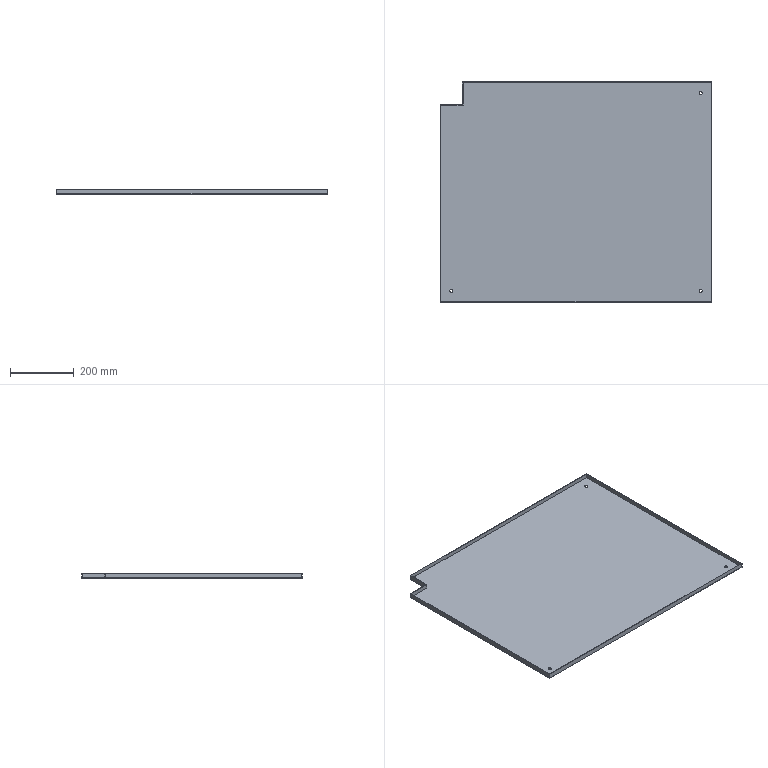Part | STEP file | 11-FGJJ-01211 | 1 solid | 21 faces | box 850 x 688 x 15 mm | volume 1239097 mm3 | plane 15 | cylinder 6 | commonest cylinder face diameters 10 x6
STEP:
#1=CARTESIAN_POINT('',(385.,-309.,2.));
#2=VERTEX_POINT('',#1);
#3=CARTESIAN_POINT('',(395.,-309.,2.));
#4=VERTEX_POINT('',#3);
#5=CARTESIAN_POINT('',(390.,-309.,2.));
#6=DIRECTION('',(0.,0.,1.));
#7=DIRECTION('',(1.,0.,0.));
#8=AXIS2_PLACEMENT_3D('',#5,#6,#7);
#9=CIRCLE('',#8,5.);
#10=EDGE_CURVE('',#2,#4,#9,.T.);
#11=ORIENTED_EDGE('',*,*,#10,.T.);
#12=CARTESIAN_POINT('',(395.,-309.,0.));
#13=VERTEX_POINT('',#12);
#14=CARTESIAN_POINT('',(395.,-309.,10.));
#15=DIRECTION('',(0.,0.,-1.));
#16=VECTOR('',#15,1000.);
#17=LINE('',#14,#16);
#18=EDGE_CURVE('',#4,#13,#17,.T.);
#19=ORIENTED_EDGE('',*,*,#18,.T.);
#20=CARTESIAN_POINT('',(385.,-309.,0.));
#21=VERTEX_POINT('',#20);
#22=CARTESIAN_POINT('',(390.,-309.,0.));
#23=DIRECTION('',(0.,0.,-1.));
#24=DIRECTION('',(-1.,0.,0.));
#25=AXIS2_PLACEMENT_3D('',#22,#23,#24);
#26=CIRCLE('',#25,5.);
#27=EDGE_CURVE('',#13,#21,#26,.T.);
#28=ORIENTED_EDGE('',*,*,#27,.T.);
#29=CARTESIAN_POINT('',(385.,-309.,10.));
#30=DIRECTION('',(0.,0.,-1.));
#31=VECTOR('',#30,1000.);
#32=LINE('',#29,#31);
#33=EDGE_CURVE('',#2,#21,#32,.T.);
#34=ORIENTED_EDGE('',*,*,#33,.F.);
#35=EDGE_LOOP('',(#11,#19,#28,#34));
#36=FACE_OUTER_BOUND('',#35,.T.);
#37=CARTESIAN_POINT('',(390.,-309.,10.));
#38=DIRECTION('',(0.,0.,-1.));
#39=DIRECTION('',(-1.,0.,0.));
#40=AXIS2_PLACEMENT_3D('',#37,#38,#39);
#41=CYLINDRICAL_SURFACE('',#40,5.);
#42=ADVANCED_FACE('',(#36),#41,.F.);
#43=CARTESIAN_POINT('',(385.,309.,0.));
#44=VERTEX_POINT('',#43);
#45=CARTESIAN_POINT('',(395.,309.,0.));
#46=VERTEX_POINT('',#45);
#47=CARTESIAN_POINT('',(390.,309.,0.));
#48=DIRECTION('',(0.,0.,1.));
#49=DIRECTION('',(1.,0.,0.));
#50=AXIS2_PLACEMENT_3D('',#47,#48,#49);
#51=CIRCLE('',#50,5.);
#52=EDGE_CURVE('',#44,#46,#51,.T.);
#53=ORIENTED_EDGE('',*,*,#52,.F.);
#54=CARTESIAN_POINT('',(385.,309.,2.));
#55=VERTEX_POINT('',#54);
#56=CARTESIAN_POINT('',(385.,309.,-8.));
#57=DIRECTION('',(0.,0.,1.));
#58=VECTOR('',#57,1000.);
#59=LINE('',#56,#58);
#60=EDGE_CURVE('',#44,#55,#59,.T.);
#61=ORIENTED_EDGE('',*,*,#60,.T.);
#62=CARTESIAN_POINT('',(395.,309.,2.));
#63=VERTEX_POINT('',#62);
#64=CARTESIAN_POINT('',(390.,309.,2.));
#65=DIRECTION('',(0.,0.,1.));
#66=DIRECTION('',(1.,0.,0.));
#67=AXIS2_PLACEMENT_3D('',#64,#65,#66);
#68=CIRCLE('',#67,5.);
#69=EDGE_CURVE('',#55,#63,#68,.T.);
#70=ORIENTED_EDGE('',*,*,#69,.T.);
#71=CARTESIAN_POINT('',(395.,309.,-8.));
#72=DIRECTION('',(0.,0.,1.));
#73=VECTOR('',#72,1000.);
#74=LINE('',#71,#73);
#75=EDGE_CURVE('',#46,#63,#74,.T.);
#76=ORIENTED_EDGE('',*,*,#75,.F.);
#77=EDGE_LOOP('',(#53,#61,#70,#76));
#78=FACE_OUTER_BOUND('',#77,.T.);
#79=CARTESIAN_POINT('',(390.,309.,-8.));
#80=DIRECTION('',(0.,0.,1.));
#81=DIRECTION('',(1.,0.,0.));
#82=AXIS2_PLACEMENT_3D('',#79,#80,#81);
#83=CYLINDRICAL_SURFACE('',#82,5.);
#84=ADVANCED_FACE('',(#78),#83,.F.);
#85=CARTESIAN_POINT('',(-395.,-309.,0.));
#86=VERTEX_POINT('',#85);
#87=CARTESIAN_POINT('',(-385.,-309.,0.));
#88=VERTEX_POINT('',#87);
#89=CARTESIAN_POINT('',(-390.,-309.,0.));
#90=DIRECTION('',(0.,0.,1.));
#91=DIRECTION('',(1.,0.,0.));
#92=AXIS2_PLACEMENT_3D('',#89,#90,#91);
#93=CIRCLE('',#92,5.);
#94=EDGE_CURVE('',#86,#88,#93,.T.);
#95=ORIENTED_EDGE('',*,*,#94,.F.);
#96=CARTESIAN_POINT('',(-395.,-309.,2.));
#97=VERTEX_POINT('',#96);
#98=CARTESIAN_POINT('',(-395.,-309.,-8.));
#99=DIRECTION('',(0.,0.,1.));
#100=VECTOR('',#99,1000.);
#101=LINE('',#98,#100);
#102=EDGE_CURVE('',#86,#97,#101,.T.);
#103=ORIENTED_EDGE('',*,*,#102,.T.);
#104=CARTESIAN_POINT('',(-385.,-309.,2.));
#105=VERTEX_POINT('',#104);
#106=CARTESIAN_POINT('',(-390.,-309.,2.));
#107=DIRECTION('',(0.,0.,1.));
#108=DIRECTION('',(1.,0.,0.));
#109=AXIS2_PLACEMENT_3D('',#106,#107,#108);
#110=CIRCLE('',#109,5.);
#111=EDGE_CURVE('',#97,#105,#110,.T.);
#112=ORIENTED_EDGE('',*,*,#111,.T.);
#113=CARTESIAN_POINT('',(-385.,-309.,-8.));
#114=DIRECTION('',(0.,0.,1.));
#115=VECTOR('',#114,1000.);
#116=LINE('',#113,#115);
#117=EDGE_CURVE('',#88,#105,#116,.T.);
#118=ORIENTED_EDGE('',*,*,#117,.F.);
#119=EDGE_LOOP('',(#95,#103,#112,#118));
#120=FACE_OUTER_BOUND('',#119,.T.);
#121=CARTESIAN_POINT('',(-390.,-309.,-8.));
#122=DIRECTION('',(0.,0.,1.));
#123=DIRECTION('',(1.,0.,0.));
#124=AXIS2_PLACEMENT_3D('',#121,#122,#123);
#125=CYLINDRICAL_SURFACE('',#124,5.);
#126=ADVANCED_FACE('',(#120),#125,.F.);
#127=CARTESIAN_POINT('',(423.,342.,15.));
#128=VERTEX_POINT('',#127);
#129=CARTESIAN_POINT('',(-353.,342.,15.));
#130=VERTEX_POINT('',#129);
#131=CARTESIAN_POINT('',(-425.,342.,15.));
#132=DIRECTION('',(-1.,0.,0.));
#133=VECTOR('',#132,1000.);
#134=LINE('',#131,#133);
#135=EDGE_CURVE('',#128,#130,#134,.T.);
#136=ORIENTED_EDGE('',*,*,#135,.T.);
#137=CARTESIAN_POINT('',(-353.,342.,2.));
#138=VERTEX_POINT('',#137);
#139=CARTESIAN_POINT('',(-353.,342.,113.995));
#140=DIRECTION('',(0.,0.,-1.));
#141=VECTOR('',#140,1000.);
#142=LINE('',#139,#141);
#143=EDGE_CURVE('',#130,#138,#142,.T.);
#144=ORIENTED_EDGE('',*,*,#143,.T.);
#145=CARTESIAN_POINT('',(423.,342.,2.));
#146=VERTEX_POINT('',#145);
#147=CARTESIAN_POINT('',(-425.,342.,2.));
#148=DIRECTION('',(-1.,0.,0.));
#149=VECTOR('',#148,1000.);
#150=LINE('',#147,#149);
#151=EDGE_CURVE('',#146,#138,#150,.T.);
#152=ORIENTED_EDGE('',*,*,#151,.F.);
#153=CARTESIAN_POINT('',(423.,342.,15.));
#154=DIRECTION('',(0.,0.,-1.));
#155=VECTOR('',#154,1000.);
#156=LINE('',#153,#155);
#157=EDGE_CURVE('',#128,#146,#156,.T.);
#158=ORIENTED_EDGE('',*,*,#157,.F.);
#159=EDGE_LOOP('',(#136,#144,#152,#158));
#160=FACE_OUTER_BOUND('',#159,.T.);
#161=CARTESIAN_POINT('',(-425.,342.,15.));
#162=DIRECTION('',(0.,-1.,0.));
#163=DIRECTION('',(0.,0.,-1.));
#164=AXIS2_PLACEMENT_3D('',#161,#162,#163);
#165=PLANE('',#164);
#166=ADVANCED_FACE('',(#160),#165,.T.);
#167=CARTESIAN_POINT('',(-423.,272.,2.));
#168=VERTEX_POINT('',#167);
#169=CARTESIAN_POINT('',(-423.,-342.,2.));
#170=VERTEX_POINT('',#169);
#171=CARTESIAN_POINT('',(-423.,344.,2.));
#172=DIRECTION('',(0.,-1.,0.));
#173=VECTOR('',#172,1000.);
#174=LINE('',#171,#173);
#175=EDGE_CURVE('',#168,#170,#174,.T.);
#176=ORIENTED_EDGE('',*,*,#175,.F.);
#177=CARTESIAN_POINT('',(-423.,272.,15.));
#178=VERTEX_POINT('',#177);
#179=CARTESIAN_POINT('',(-423.,272.,113.995));
#180=DIRECTION('',(0.,0.,-1.));
#181=VECTOR('',#180,1000.);
#182=LINE('',#179,#181);
#183=EDGE_CURVE('',#178,#168,#182,.T.);
#184=ORIENTED_EDGE('',*,*,#183,.F.);
#185=CARTESIAN_POINT('',(-423.,-342.,15.));
#186=VERTEX_POINT('',#185);
#187=CARTESIAN_POINT('',(-423.,344.,15.));
#188=DIRECTION('',(0.,-1.,0.));
#189=VECTOR('',#188,1000.);
#190=LINE('',#187,#189);
#191=EDGE_CURVE('',#178,#186,#190,.T.);
#192=ORIENTED_EDGE('',*,*,#191,.T.);
#193=CARTESIAN_POINT('',(-423.,-342.,15.));
#194=DIRECTION('',(0.,0.,-1.));
#195=VECTOR('',#194,1000.);
#196=LINE('',#193,#195);
#197=EDGE_CURVE('',#186,#170,#196,.T.);
#198=ORIENTED_EDGE('',*,*,#197,.T.);
#199=EDGE_LOOP('',(#176,#184,#192,#198));
#200=FACE_OUTER_BOUND('',#199,.T.);
#201=CARTESIAN_POINT('',(-423.,344.,15.));
#202=DIRECTION('',(1.,0.,0.));
#203=DIRECTION('',(0.,1.,0.));
#204=AXIS2_PLACEMENT_3D('',#201,#202,#203);
#205=PLANE('',#204);
#206=ADVANCED_FACE('',(#200),#205,.T.);
#207=ORIENTED_EDGE('',*,*,#10,.F.);
#208=CARTESIAN_POINT('',(390.,-309.,2.));
#209=DIRECTION('',(0.,0.,1.));
#210=DIRECTION('',(1.,0.,0.));
#211=AXIS2_PLACEMENT_3D('',#208,#209,#210);
#212=CIRCLE('',#211,5.);
#213=EDGE_CURVE('',#4,#2,#212,.T.);
#214=ORIENTED_EDGE('',*,*,#213,.F.);
#215=EDGE_LOOP('',(#207,#214));
#216=FACE_BOUND('',#215,.T.);
#217=CARTESIAN_POINT('',(390.,309.,2.));
#218=DIRECTION('',(0.,0.,1.));
#219=DIRECTION('',(1.,0.,0.));
#220=AXIS2_PLACEMENT_3D('',#217,#218,#219);
#221=CIRCLE('',#220,5.);
#222=EDGE_CURVE('',#63,#55,#221,.T.);
#223=ORIENTED_EDGE('',*,*,#222,.F.);
#224=ORIENTED_EDGE('',*,*,#69,.F.);
#225=EDGE_LOOP('',(#223,#224));
#226=FACE_BOUND('',#225,.T.);
#227=CARTESIAN_POINT('',(-390.,-309.,2.));
#228=DIRECTION('',(0.,0.,1.));
#229=DIRECTION('',(1.,0.,0.));
#230=AXIS2_PLACEMENT_3D('',#227,#228,#229);
#231=CIRCLE('',#230,5.);
#232=EDGE_CURVE('',#105,#97,#231,.T.);
#233=ORIENTED_EDGE('',*,*,#232,.F.);
#234=ORIENTED_EDGE('',*,*,#111,.F.);
#235=EDGE_LOOP('',(#233,#234));
#236=FACE_BOUND('',#235,.T.);
#237=CARTESIAN_POINT('',(-353.,272.,2.));
#238=VERTEX_POINT('',#237);
#239=CARTESIAN_POINT('',(-353.,342.,2.));
#240=DIRECTION('',(0.,1.,0.));
#241=VECTOR('',#240,1000.);
#242=LINE('',#239,#241);
#243=EDGE_CURVE('',#238,#138,#242,.T.);
#244=ORIENTED_EDGE('',*,*,#243,.F.);
#245=CARTESIAN_POINT('',(-423.,272.,2.));
#246=DIRECTION('',(1.,0.,0.));
#247=VECTOR('',#246,1000.);
#248=LINE('',#245,#247);
#249=EDGE_CURVE('',#168,#238,#248,.T.);
#250=ORIENTED_EDGE('',*,*,#249,.F.);
#251=ORIENTED_EDGE('',*,*,#175,.T.);
#252=CARTESIAN_POINT('',(423.,-342.,2.));
#253=VERTEX_POINT('',#252);
#254=CARTESIAN_POINT('',(-425.,-342.,2.));
#255=DIRECTION('',(1.,0.,0.));
#256=VECTOR('',#255,1000.);
#257=LINE('',#254,#256);
#258=EDGE_CURVE('',#170,#253,#257,.T.);
#259=ORIENTED_EDGE('',*,*,#258,.T.);
#260=CARTESIAN_POINT('',(423.,344.,2.));
#261=DIRECTION('',(0.,1.,0.));
#262=VECTOR('',#261,1000.);
#263=LINE('',#260,#262);
#264=EDGE_CURVE('',#253,#146,#263,.T.);
#265=ORIENTED_EDGE('',*,*,#264,.T.);
#266=ORIENTED_EDGE('',*,*,#151,.T.);
#267=EDGE_LOOP('',(#244,#250,#251,#259,#265,#266));
#268=FACE_OUTER_BOUND('',#267,.T.);
#269=CARTESIAN_POINT('',(0.,0.,2.));
#270=DIRECTION('',(0.,0.,1.));
#271=DIRECTION('',(1.,0.,0.));
#272=AXIS2_PLACEMENT_3D('',#269,#270,#271);
#273=PLANE('',#272);
#274=ADVANCED_FACE('',(#216,#226,#236,#268),#273,.T.);
#275=CARTESIAN_POINT('',(425.,-344.,0.));
#276=VERTEX_POINT('',#275);
#277=CARTESIAN_POINT('',(425.,344.,0.));
#278=VERTEX_POINT('',#277);
#279=CARTESIAN_POINT('',(425.,344.,0.));
#280=DIRECTION('',(0.,1.,0.));
#281=VECTOR('',#280,1000.);
#282=LINE('',#279,#281);
#283=EDGE_CURVE('',#276,#278,#282,.T.);
#284=ORIENTED_EDGE('',*,*,#283,.T.);
#285=CARTESIAN_POINT('',(425.,344.,15.));
#286=VERTEX_POINT('',#285);
#287=CARTESIAN_POINT('',(425.,344.,15.));
#288=DIRECTION('',(0.,0.,-1.));
#289=VECTOR('',#288,1000.);
#290=LINE('',#287,#289);
#291=EDGE_CURVE('',#286,#278,#290,.T.);
#292=ORIENTED_EDGE('',*,*,#291,.F.);
#293=CARTESIAN_POINT('',(425.,-344.,15.));
#294=VERTEX_POINT('',#293);
#295=CARTESIAN_POINT('',(425.,344.,15.));
#296=DIRECTION('',(0.,1.,0.));
#297=VECTOR('',#296,1000.);
#298=LINE('',#295,#297);
#299=EDGE_CURVE('',#294,#286,#298,.T.);
#300=ORIENTED_EDGE('',*,*,#299,.F.);
#301=CARTESIAN_POINT('',(425.,-344.,15.));
#302=DIRECTION('',(0.,0.,-1.));
#303=VECTOR('',#302,1000.);
#304=LINE('',#301,#303);
#305=EDGE_CURVE('',#294,#276,#304,.T.);
#306=ORIENTED_EDGE('',*,*,#305,.T.);
#307=EDGE_LOOP('',(#284,#292,#300,#306));
#308=FACE_OUTER_BOUND('',#307,.T.);
#309=CARTESIAN_POINT('',(425.,344.,15.));
#310=DIRECTION('',(-1.,0.,0.));
#311=DIRECTION('',(0.,-1.,0.));
#312=AXIS2_PLACEMENT_3D('',#309,#310,#311);
#313=PLANE('',#312);
#314=ADVANCED_FACE('',(#308),#313,.F.);
#315=CARTESIAN_POINT('',(-355.,344.,0.));
#316=VERTEX_POINT('',#315);
#317=CARTESIAN_POINT('',(-425.,344.,0.));
#318=DIRECTION('',(-1.,0.,0.));
#319=VECTOR('',#318,1000.);
#320=LINE('',#317,#319);
#321=EDGE_CURVE('',#278,#316,#320,.T.);
#322=ORIENTED_EDGE('',*,*,#321,.T.);
#323=CARTESIAN_POINT('',(-355.,344.,15.));
#324=VERTEX_POINT('',#323);
#325=CARTESIAN_POINT('',(-355.,344.,26.));
#326=DIRECTION('',(0.,0.,-1.));
#327=VECTOR('',#326,1000.);
#328=LINE('',#325,#327);
#329=EDGE_CURVE('',#324,#316,#328,.T.);
#330=ORIENTED_EDGE('',*,*,#329,.F.);
#331=CARTESIAN_POINT('',(-425.,344.,15.));
#332=DIRECTION('',(-1.,0.,0.));
#333=VECTOR('',#332,1000.);
#334=LINE('',#331,#333);
#335=EDGE_CURVE('',#286,#324,#334,.T.);
#336=ORIENTED_EDGE('',*,*,#335,.F.);
#337=ORIENTED_EDGE('',*,*,#291,.T.);
#338=EDGE_LOOP('',(#322,#330,#336,#337));
#339=FACE_OUTER_BOUND('',#338,.T.);
#340=CARTESIAN_POINT('',(-425.,344.,15.));
#341=DIRECTION('',(0.,-1.,0.));
#342=DIRECTION('',(0.,0.,-1.));
#343=AXIS2_PLACEMENT_3D('',#340,#341,#342);
#344=PLANE('',#343);
#345=ADVANCED_FACE('',(#339),#344,.F.);
#346=CARTESIAN_POINT('',(-425.,274.,15.));
#347=VERTEX_POINT('',#346);
#348=CARTESIAN_POINT('',(-425.,-344.,15.));
#349=VERTEX_POINT('',#348);
#350=CARTESIAN_POINT('',(-425.,344.,15.));
#351=DIRECTION('',(0.,-1.,0.));
#352=VECTOR('',#351,1000.);
#353=LINE('',#350,#352);
#354=EDGE_CURVE('',#347,#349,#353,.T.);
#355=ORIENTED_EDGE('',*,*,#354,.F.);
#356=CARTESIAN_POINT('',(-425.,274.,0.));
#357=VERTEX_POINT('',#356);
#358=CARTESIAN_POINT('',(-425.,274.,26.));
#359=DIRECTION('',(0.,0.,-1.));
#360=VECTOR('',#359,1000.);
#361=LINE('',#358,#360);
#362=EDGE_CURVE('',#347,#357,#361,.T.);
#363=ORIENTED_EDGE('',*,*,#362,.T.);
#364=CARTESIAN_POINT('',(-425.,-344.,0.));
#365=VERTEX_POINT('',#364);
#366=CARTESIAN_POINT('',(-425.,344.,0.));
#367=DIRECTION('',(0.,-1.,0.));
#368=VECTOR('',#367,1000.);
#369=LINE('',#366,#368);
#370=EDGE_CURVE('',#357,#365,#369,.T.);
#371=ORIENTED_EDGE('',*,*,#370,.T.);
#372=CARTESIAN_POINT('',(-425.,-344.,15.));
#373=DIRECTION('',(0.,0.,-1.));
#374=VECTOR('',#373,1000.);
#375=LINE('',#372,#374);
#376=EDGE_CURVE('',#349,#365,#375,.T.);
#377=ORIENTED_EDGE('',*,*,#376,.F.);
#378=EDGE_LOOP('',(#355,#363,#371,#377));
#379=FACE_OUTER_BOUND('',#378,.T.);
#380=CARTESIAN_POINT('',(-425.,344.,15.));
#381=DIRECTION('',(1.,0.,0.));
#382=DIRECTION('',(0.,1.,0.));
#383=AXIS2_PLACEMENT_3D('',#380,#381,#382);
#384=PLANE('',#383);
#385=ADVANCED_FACE('',(#379),#384,.F.);
#386=CARTESIAN_POINT('',(-425.,-344.,0.));
#387=DIRECTION('',(1.,0.,0.));
#388=VECTOR('',#387,1000.);
#389=LINE('',#386,#388);
#390=EDGE_CURVE('',#365,#276,#389,.T.);
#391=ORIENTED_EDGE('',*,*,#390,.T.);
#392=ORIENTED_EDGE('',*,*,#305,.F.);
#393=CARTESIAN_POINT('',(-425.,-344.,15.));
#394=DIRECTION('',(1.,0.,0.));
#395=VECTOR('',#394,1000.);
#396=LINE('',#393,#395);
#397=EDGE_CURVE('',#349,#294,#396,.T.);
#398=ORIENTED_EDGE('',*,*,#397,.F.);
#399=ORIENTED_EDGE('',*,*,#376,.T.);
#400=EDGE_LOOP('',(#391,#392,#398,#399));
#401=FACE_OUTER_BOUND('',#400,.T.);
#402=CARTESIAN_POINT('',(-425.,-344.,15.));
#403=DIRECTION('',(0.,1.,0.));
#404=DIRECTION('',(0.,0.,1.));
#405=AXIS2_PLACEMENT_3D('',#402,#403,#404);
#406=PLANE('',#405);
#407=ADVANCED_FACE('',(#401),#406,.F.);
#408=CARTESIAN_POINT('',(-355.,274.,15.));
#409=VERTEX_POINT('',#408);
#410=CARTESIAN_POINT('',(-355.,0.,15.));
#411=DIRECTION('',(0.,1.,0.));
#412=VECTOR('',#411,1000.);
#413=LINE('',#410,#412);
#414=EDGE_CURVE('',#409,#324,#413,.T.);
#415=ORIENTED_EDGE('',*,*,#414,.F.);
#416=CARTESIAN_POINT('',(0.,274.,15.));
#417=DIRECTION('',(1.,0.,0.));
#418=VECTOR('',#417,1000.);
#419=LINE('',#416,#418);
#420=EDGE_CURVE('',#347,#409,#419,.T.);
#421=ORIENTED_EDGE('',*,*,#420,.F.);
#422=ORIENTED_EDGE('',*,*,#354,.T.);
#423=ORIENTED_EDGE('',*,*,#397,.T.);
#424=ORIENTED_EDGE('',*,*,#299,.T.);
#425=ORIENTED_EDGE('',*,*,#335,.T.);
#426=EDGE_LOOP('',(#415,#421,#422,#423,#424,#425));
#427=FACE_OUTER_BOUND('',#426,.T.);
#428=CARTESIAN_POINT('',(-353.,272.,15.));
#429=VERTEX_POINT('',#428);
#430=CARTESIAN_POINT('',(-353.,342.,15.));
#431=DIRECTION('',(0.,1.,0.));
#432=VECTOR('',#431,1000.);
#433=LINE('',#430,#432);
#434=EDGE_CURVE('',#429,#130,#433,.T.);
#435=ORIENTED_EDGE('',*,*,#434,.T.);
#436=ORIENTED_EDGE('',*,*,#135,.F.);
#437=CARTESIAN_POINT('',(423.,-342.,15.));
#438=VERTEX_POINT('',#437);
#439=CARTESIAN_POINT('',(423.,344.,15.));
#440=DIRECTION('',(0.,1.,0.));
#441=VECTOR('',#440,1000.);
#442=LINE('',#439,#441);
#443=EDGE_CURVE('',#438,#128,#442,.T.);
#444=ORIENTED_EDGE('',*,*,#443,.F.);
#445=CARTESIAN_POINT('',(-425.,-342.,15.));
#446=DIRECTION('',(1.,0.,0.));
#447=VECTOR('',#446,1000.);
#448=LINE('',#445,#447);
#449=EDGE_CURVE('',#186,#438,#448,.T.);
#450=ORIENTED_EDGE('',*,*,#449,.F.);
#451=ORIENTED_EDGE('',*,*,#191,.F.);
#452=CARTESIAN_POINT('',(-423.,272.,15.));
#453=DIRECTION('',(1.,0.,0.));
#454=VECTOR('',#453,1000.);
#455=LINE('',#452,#454);
#456=EDGE_CURVE('',#178,#429,#455,.T.);
#457=ORIENTED_EDGE('',*,*,#456,.T.);
#458=EDGE_LOOP('',(#435,#436,#444,#450,#451,#457));
#459=FACE_BOUND('',#458,.T.);
#460=CARTESIAN_POINT('',(0.,0.,15.));
#461=DIRECTION('',(0.,0.,1.));
#462=DIRECTION('',(1.,0.,0.));
#463=AXIS2_PLACEMENT_3D('',#460,#461,#462);
#464=PLANE('',#463);
#465=ADVANCED_FACE('',(#427,#459),#464,.T.);
#466=CARTESIAN_POINT('',(390.,-309.,0.));
#467=DIRECTION('',(0.,0.,-1.));
#468=DIRECTION('',(-1.,0.,0.));
#469=AXIS2_PLACEMENT_3D('',#466,#467,#468);
#470=CIRCLE('',#469,5.);
#471=EDGE_CURVE('',#21,#13,#470,.T.);
#472=ORIENTED_EDGE('',*,*,#471,.F.);
#473=ORIENTED_EDGE('',*,*,#27,.F.);
#474=EDGE_LOOP('',(#472,#473));
#475=FACE_BOUND('',#474,.T.);
#476=CARTESIAN_POINT('',(390.,309.,0.));
#477=DIRECTION('',(0.,0.,1.));
#478=DIRECTION('',(1.,0.,0.));
#479=AXIS2_PLACEMENT_3D('',#476,#477,#478);
#480=CIRCLE('',#479,5.);
#481=EDGE_CURVE('',#46,#44,#480,.T.);
#482=ORIENTED_EDGE('',*,*,#481,.T.);
#483=ORIENTED_EDGE('',*,*,#52,.T.);
#484=EDGE_LOOP('',(#482,#483));
#485=FACE_BOUND('',#484,.T.);
#486=CARTESIAN_POINT('',(-390.,-309.,0.));
#487=DIRECTION('',(0.,0.,1.));
#488=DIRECTION('',(1.,0.,0.));
#489=AXIS2_PLACEMENT_3D('',#486,#487,#488);
#490=CIRCLE('',#489,5.);
#491=EDGE_CURVE('',#88,#86,#490,.T.);
#492=ORIENTED_EDGE('',*,*,#491,.T.);
#493=ORIENTED_EDGE('',*,*,#94,.T.);
#494=EDGE_LOOP('',(#492,#493));
#495=FACE_BOUND('',#494,.T.);
#496=ORIENTED_EDGE('',*,*,#370,.F.);
#497=CARTESIAN_POINT('',(-355.,274.,0.));
#498=VERTEX_POINT('',#497);
#499=CARTESIAN_POINT('',(-425.,274.,0.));
#500=DIRECTION('',(-1.,0.,0.));
#501=VECTOR('',#500,1000.);
#502=LINE('',#499,#501);
#503=EDGE_CURVE('',#498,#357,#502,.T.);
#504=ORIENTED_EDGE('',*,*,#503,.F.);
#505=CARTESIAN_POINT('',(-355.,344.,0.));
#506=DIRECTION('',(0.,-1.,0.));
#507=VECTOR('',#506,1000.);
#508=LINE('',#505,#507);
#509=EDGE_CURVE('',#316,#498,#508,.T.);
#510=ORIENTED_EDGE('',*,*,#509,.F.);
#511=ORIENTED_EDGE('',*,*,#321,.F.);
#512=ORIENTED_EDGE('',*,*,#283,.F.);
#513=ORIENTED_EDGE('',*,*,#390,.F.);
#514=EDGE_LOOP('',(#496,#504,#510,#511,#512,#513));
#515=FACE_OUTER_BOUND('',#514,.T.);
#516=CARTESIAN_POINT('',(0.,0.,0.));
#517=DIRECTION('',(0.,0.,1.));
#518=DIRECTION('',(1.,0.,0.));
#519=AXIS2_PLACEMENT_3D('',#516,#517,#518);
#520=PLANE('',#519);
#521=ADVANCED_FACE('',(#475,#485,#495,#515),#520,.F.);
#522=ORIENTED_EDGE('',*,*,#264,.F.);
#523=CARTESIAN_POINT('',(423.,-342.,15.));
#524=DIRECTION('',(0.,0.,-1.));
#525=VECTOR('',#524,1000.);
#526=LINE('',#523,#525);
#527=EDGE_CURVE('',#438,#253,#526,.T.);
#528=ORIENTED_EDGE('',*,*,#527,.F.);
#529=ORIENTED_EDGE('',*,*,#443,.T.);
#530=ORIENTED_EDGE('',*,*,#157,.T.);
#531=EDGE_LOOP('',(#522,#528,#529,#530));
#532=FACE_OUTER_BOUND('',#531,.T.);
#533=CARTESIAN_POINT('',(423.,344.,15.));
#534=DIRECTION('',(-1.,0.,0.));
#535=DIRECTION('',(0.,-1.,0.));
#536=AXIS2_PLACEMENT_3D('',#533,#534,#535);
#537=PLANE('',#536);
#538=ADVANCED_FACE('',(#532),#537,.T.);
#539=ORIENTED_EDGE('',*,*,#258,.F.);
#540=ORIENTED_EDGE('',*,*,#197,.F.);
#541=ORIENTED_EDGE('',*,*,#449,.T.);
#542=ORIENTED_EDGE('',*,*,#527,.T.);
#543=EDGE_LOOP('',(#539,#540,#541,#542));
#544=FACE_OUTER_BOUND('',#543,.T.);
#545=CARTESIAN_POINT('',(-425.,-342.,15.));
#546=DIRECTION('',(0.,1.,0.));
#547=DIRECTION('',(0.,0.,1.));
#548=AXIS2_PLACEMENT_3D('',#545,#546,#547);
#549=PLANE('',#548);
#550=ADVANCED_FACE('',(#544),#549,.T.);
#551=ORIENTED_EDGE('',*,*,#102,.F.);
#552=ORIENTED_EDGE('',*,*,#491,.F.);
#553=ORIENTED_EDGE('',*,*,#117,.T.);
#554=ORIENTED_EDGE('',*,*,#232,.T.);
#555=EDGE_LOOP('',(#551,#552,#553,#554));
#556=FACE_OUTER_BOUND('',#555,.T.);
#557=CARTESIAN_POINT('',(-390.,-309.,-8.));
#558=DIRECTION('',(0.,0.,1.));
#559=DIRECTION('',(1.,0.,0.));
#560=AXIS2_PLACEMENT_3D('',#557,#558,#559);
#561=CYLINDRICAL_SURFACE('',#560,5.);
#562=ADVANCED_FACE('',(#556),#561,.F.);
#563=ORIENTED_EDGE('',*,*,#60,.F.);
#564=ORIENTED_EDGE('',*,*,#481,.F.);
#565=ORIENTED_EDGE('',*,*,#75,.T.);
#566=ORIENTED_EDGE('',*,*,#222,.T.);
#567=EDGE_LOOP('',(#563,#564,#565,#566));
#568=FACE_OUTER_BOUND('',#567,.T.);
#569=CARTESIAN_POINT('',(390.,309.,-8.));
#570=DIRECTION('',(0.,0.,1.));
#571=DIRECTION('',(1.,0.,0.));
#572=AXIS2_PLACEMENT_3D('',#569,#570,#571);
#573=CYLINDRICAL_SURFACE('',#572,5.);
#574=ADVANCED_FACE('',(#568),#573,.F.);
#575=ORIENTED_EDGE('',*,*,#420,.T.);
#576=CARTESIAN_POINT('',(-355.,274.,26.));
#577=DIRECTION('',(0.,0.,-1.));
#578=VECTOR('',#577,1000.);
#579=LINE('',#576,#578);
#580=EDGE_CURVE('',#409,#498,#579,.T.);
#581=ORIENTED_EDGE('',*,*,#580,.T.);
#582=ORIENTED_EDGE('',*,*,#503,.T.);
#583=ORIENTED_EDGE('',*,*,#362,.F.);
#584=EDGE_LOOP('',(#575,#581,#582,#583));
#585=FACE_OUTER_BOUND('',#584,.T.);
#586=CARTESIAN_POINT('',(-425.,274.,26.));
#587=DIRECTION('',(0.,-1.,0.));
#588=DIRECTION('',(0.,0.,-1.));
#589=AXIS2_PLACEMENT_3D('',#586,#587,#588);
#590=PLANE('',#589);
#591=ADVANCED_FACE('',(#585),#590,.F.);
#592=ORIENTED_EDGE('',*,*,#580,.F.);
#593=ORIENTED_EDGE('',*,*,#414,.T.);
#594=ORIENTED_EDGE('',*,*,#329,.T.);
#595=ORIENTED_EDGE('',*,*,#509,.T.);
#596=EDGE_LOOP('',(#592,#593,#594,#595));
#597=FACE_OUTER_BOUND('',#596,.T.);
#598=CARTESIAN_POINT('',(-355.,344.,26.));
#599=DIRECTION('',(1.,0.,0.));
#600=DIRECTION('',(0.,0.,-1.));
#601=AXIS2_PLACEMENT_3D('',#598,#599,#600);
#602=PLANE('',#601);
#603=ADVANCED_FACE('',(#597),#602,.F.);
#604=ORIENTED_EDGE('',*,*,#456,.F.);
#605=ORIENTED_EDGE('',*,*,#183,.T.);
#606=ORIENTED_EDGE('',*,*,#249,.T.);
#607=CARTESIAN_POINT('',(-353.,272.,113.995));
#608=DIRECTION('',(0.,0.,-1.));
#609=VECTOR('',#608,1000.);
#610=LINE('',#607,#609);
#611=EDGE_CURVE('',#429,#238,#610,.T.);
#612=ORIENTED_EDGE('',*,*,#611,.F.);
#613=EDGE_LOOP('',(#604,#605,#606,#612));
#614=FACE_OUTER_BOUND('',#613,.T.);
#615=CARTESIAN_POINT('',(-423.,272.,113.995));
#616=DIRECTION('',(0.,1.,0.));
#617=DIRECTION('',(0.,0.,1.));
#618=AXIS2_PLACEMENT_3D('',#615,#616,#617);
#619=PLANE('',#618);
#620=ADVANCED_FACE('',(#614),#619,.F.);
#621=ORIENTED_EDGE('',*,*,#434,.F.);
#622=ORIENTED_EDGE('',*,*,#611,.T.);
#623=ORIENTED_EDGE('',*,*,#243,.T.);
#624=ORIENTED_EDGE('',*,*,#143,.F.);
#625=EDGE_LOOP('',(#621,#622,#623,#624));
#626=FACE_OUTER_BOUND('',#625,.T.);
#627=CARTESIAN_POINT('',(-353.,342.,113.995));
#628=DIRECTION('',(-1.,0.,0.));
#629=DIRECTION('',(0.,0.,1.));
#630=AXIS2_PLACEMENT_3D('',#627,#628,#629);
#631=PLANE('',#630);
#632=ADVANCED_FACE('',(#626),#631,.F.);
#633=ORIENTED_EDGE('',*,*,#18,.F.);
#634=ORIENTED_EDGE('',*,*,#213,.T.);
#635=ORIENTED_EDGE('',*,*,#33,.T.);
#636=ORIENTED_EDGE('',*,*,#471,.T.);
#637=EDGE_LOOP('',(#633,#634,#635,#636));
#638=FACE_OUTER_BOUND('',#637,.T.);
#639=CARTESIAN_POINT('',(390.,-309.,10.));
#640=DIRECTION('',(0.,0.,-1.));
#641=DIRECTION('',(-1.,0.,0.));
#642=AXIS2_PLACEMENT_3D('',#639,#640,#641);
#643=CYLINDRICAL_SURFACE('',#642,5.);
#644=ADVANCED_FACE('',(#638),#643,.F.);
#645=CLOSED_SHELL('',(#42,#84,#126,#166,#206,#274,#314,#345,#385,#407,#465,#521,#538,#550,#562,#574,#591,#603,#620,#632,#644));
#646=MANIFOLD_SOLID_BREP('',#645);
#647=CARTESIAN_POINT('',(0.,0.,0.));
#648=DIRECTION('',(0.,0.,1.));
#649=DIRECTION('',(1.,0.,0.));
#650=AXIS2_PLACEMENT_3D('',#647,#648,#649);
#651=(LENGTH_UNIT()NAMED_UNIT(*)SI_UNIT(.MILLI.,.METRE.));
#652=UNCERTAINTY_MEASURE_WITH_UNIT(LENGTH_MEASURE(0.00001),#651,'','');
#653=(NAMED_UNIT(*)PLANE_ANGLE_UNIT()SI_UNIT($,.RADIAN.));
#654=(NAMED_UNIT(*)SI_UNIT($,.STERADIAN.)SOLID_ANGLE_UNIT());
#655=(GEOMETRIC_REPRESENTATION_CONTEXT(3)GLOBAL_UNCERTAINTY_ASSIGNED_CONTEXT((#652))GLOBAL_UNIT_ASSIGNED_CONTEXT((#651,#653,#654))REPRESENTATION_CONTEXT('',''));
#656=ADVANCED_BREP_SHAPE_REPRESENTATION('',(#646,#650),#655);